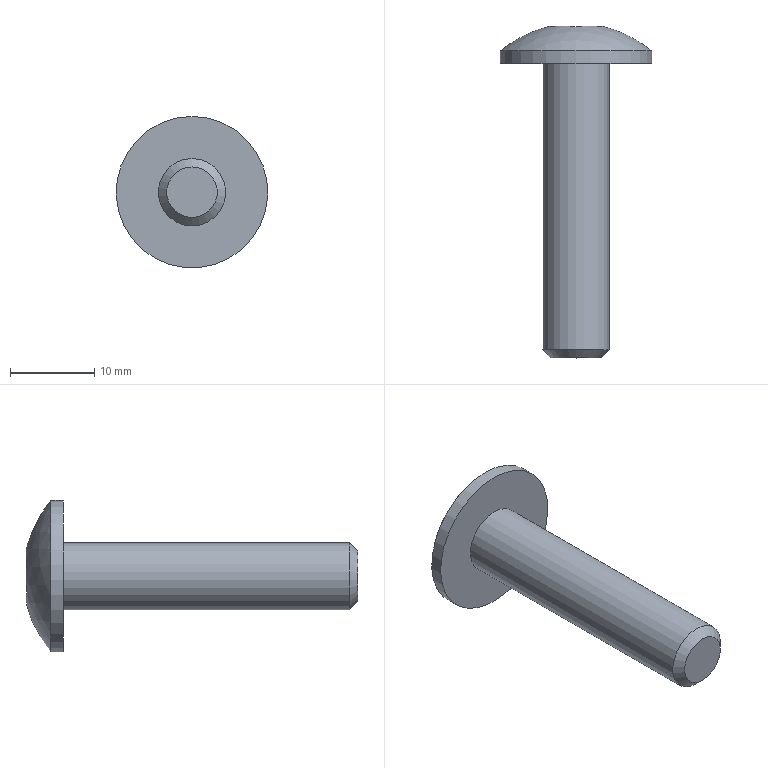Part | STEP file | PN_0012 | 1 solid | 13 faces | box 18 x 39.451 x 18 mm | volume 2453 mm3 | plane 9 | cylinder 2 | sphere 1 | cone 1 | commonest cylinder face diameters 8 x1 18 x1
STEP:
#1=CARTESIAN_POINT('',(0.,0.,0.));
#2=DIRECTION('',(0.,0.,1.));
#3=DIRECTION('',(1.,0.,0.));
#4=AXIS2_PLACEMENT_3D('',#1,#2,#3);
#5=CARTESIAN_POINT('',(0.,0.,9.));
#6=VERTEX_POINT('',#5);
#7=CARTESIAN_POINT('',(0.,0.,0.));
#8=DIRECTION('',(0.,1.,0.));
#9=DIRECTION('',(0.,0.,1.));
#10=AXIS2_PLACEMENT_3D('',#7,#8,#9);
#11=CIRCLE('',#10,9.);
#12=CARTESIAN_POINT('',(0.,0.,0.));
#13=DIRECTION('',(0.,1.,0.));
#14=DIRECTION('',(0.,0.,1.));
#15=AXIS2_PLACEMENT_3D('',#12,#13,#14);
#16=PLANE('',#15);
#17=CARTESIAN_POINT('',(0.,0.));
#18=DIRECTION('',(1.,0.));
#19=AXIS2_PLACEMENT_2D('',#17,#18);
#20=CIRCLE('',#19,9.);
#21=(GEOMETRIC_REPRESENTATION_CONTEXT(2)PARAMETRIC_REPRESENTATION_CONTEXT()REPRESENTATION_CONTEXT('',''));
#22=DEFINITIONAL_REPRESENTATION('',(#20),#21);
#23=PCURVE('',#16,#22);
#24=CARTESIAN_POINT('',(0.,70.,0.));
#25=DIRECTION('',(0.,1.,0.));
#26=DIRECTION('',(0.,0.,1.));
#27=AXIS2_PLACEMENT_3D('',#24,#25,#26);
#28=CYLINDRICAL_SURFACE('',#27,9.);
#29=CARTESIAN_POINT('',(0.,-70.));
#30=DIRECTION('',(1.,0.));
#31=VECTOR('',#30,1.);
#32=LINE('',#29,#31);
#33=(GEOMETRIC_REPRESENTATION_CONTEXT(2)PARAMETRIC_REPRESENTATION_CONTEXT()REPRESENTATION_CONTEXT('',''));
#34=DEFINITIONAL_REPRESENTATION('',(#32),#33);
#35=PCURVE('',#28,#34);
#36=SURFACE_CURVE('',#11,(#23,#35),.PCURVE_S1.);
#37=EDGE_CURVE('',#6,#6,#36,.T.);
#38=ORIENTED_EDGE('',*,*,#37,.F.);
#39=EDGE_LOOP('',(#38));
#40=FACE_BOUND('',#39,.T.);
#41=CARTESIAN_POINT('',(0.,0.,4.));
#42=VERTEX_POINT('',#41);
#43=CARTESIAN_POINT('',(0.,0.,0.));
#44=DIRECTION('',(0.,-1.,0.));
#45=DIRECTION('',(0.,0.,1.));
#46=AXIS2_PLACEMENT_3D('',#43,#44,#45);
#47=CIRCLE('',#46,4.);
#48=CARTESIAN_POINT('',(4.,0.));
#49=CARTESIAN_POINT('',(4.,-6.928));
#50=CARTESIAN_POINT('',(-2.,-3.464));
#51=CARTESIAN_POINT('',(-8.,0.));
#52=CARTESIAN_POINT('',(-2.,3.464));
#53=CARTESIAN_POINT('',(4.,6.928));
#54=CARTESIAN_POINT('',(4.,0.));
#55=(BOUNDED_CURVE()B_SPLINE_CURVE(2,(#48,#49,#50,#51,#52,#53,#54),.UNSPECIFIED.,.T.,.F.)B_SPLINE_CURVE_WITH_KNOTS((1,2,2,2,2,1),(-2.094,0.,2.094,4.189,6.283,8.378),.UNSPECIFIED.)CURVE()GEOMETRIC_REPRESENTATION_ITEM()RATIONAL_B_SPLINE_CURVE((1.,0.5,1.,0.5,1.,0.5,1.))REPRESENTATION_ITEM(''));
#56=(GEOMETRIC_REPRESENTATION_CONTEXT(2)PARAMETRIC_REPRESENTATION_CONTEXT()REPRESENTATION_CONTEXT('',''));
#57=DEFINITIONAL_REPRESENTATION('',(#55),#56);
#58=PCURVE('',#16,#57);
#59=CARTESIAN_POINT('',(0.,-35.,0.));
#60=DIRECTION('',(0.,1.,0.));
#61=DIRECTION('',(0.,0.,1.));
#62=AXIS2_PLACEMENT_3D('',#59,#60,#61);
#63=CYLINDRICAL_SURFACE('',#62,4.);
#64=CARTESIAN_POINT('',(6.283,35.));
#65=DIRECTION('',(-1.,0.));
#66=VECTOR('',#65,1.);
#67=LINE('',#64,#66);
#68=(GEOMETRIC_REPRESENTATION_CONTEXT(2)PARAMETRIC_REPRESENTATION_CONTEXT()REPRESENTATION_CONTEXT('',''));
#69=DEFINITIONAL_REPRESENTATION('',(#67),#68);
#70=PCURVE('',#63,#69);
#71=SURFACE_CURVE('',#47,(#58,#70),.PCURVE_S1.);
#72=EDGE_CURVE('',#42,#42,#71,.T.);
#73=ORIENTED_EDGE('',*,*,#72,.F.);
#74=EDGE_LOOP('',(#73));
#75=FACE_BOUND('',#74,.T.);
#76=ADVANCED_FACE('',(#40,#75),#16,.F.);
#77=CARTESIAN_POINT('',(0.,1.5,9.));
#78=VERTEX_POINT('',#77);
#79=CARTESIAN_POINT('',(0.,1.5,0.));
#80=DIRECTION('',(0.,1.,0.));
#81=DIRECTION('',(0.,0.,1.));
#82=AXIS2_PLACEMENT_3D('',#79,#80,#81);
#83=CIRCLE('',#82,9.);
#84=CARTESIAN_POINT('',(0.,-9.224,0.));
#85=DIRECTION('',(0.,0.,-1.));
#86=DIRECTION('',(1.,0.,0.));
#87=AXIS2_PLACEMENT_3D('',#84,#85,#86);
#88=SPHERICAL_SURFACE('',#87,14.);
#89=CARTESIAN_POINT('',(4.712,-0.6982));
#90=CARTESIAN_POINT('',(4.794,-0.6988));
#91=CARTESIAN_POINT('',(4.951,-0.6746));
#92=CARTESIAN_POINT('',(5.148,-0.5787));
#93=CARTESIAN_POINT('',(5.286,-0.4389));
#94=CARTESIAN_POINT('',(5.372,-0.2727));
#95=CARTESIAN_POINT('',(5.412,-0.09234));
#96=CARTESIAN_POINT('',(5.412,0.09234));
#97=CARTESIAN_POINT('',(5.372,0.2727));
#98=CARTESIAN_POINT('',(5.286,0.439));
#99=CARTESIAN_POINT('',(5.148,0.5786));
#100=CARTESIAN_POINT('',(4.952,0.6749));
#101=CARTESIAN_POINT('',(4.712,0.7099));
#102=CARTESIAN_POINT('',(4.473,0.6749));
#103=CARTESIAN_POINT('',(4.277,0.5786));
#104=CARTESIAN_POINT('',(4.138,0.439));
#105=CARTESIAN_POINT('',(4.053,0.2727));
#106=CARTESIAN_POINT('',(4.012,0.09234));
#107=CARTESIAN_POINT('',(4.012,-0.09234));
#108=CARTESIAN_POINT('',(4.053,-0.2727));
#109=CARTESIAN_POINT('',(4.138,-0.4389));
#110=CARTESIAN_POINT('',(4.277,-0.5787));
#111=CARTESIAN_POINT('',(4.474,-0.6746));
#112=CARTESIAN_POINT('',(4.63,-0.6988));
#113=CARTESIAN_POINT('',(4.712,-0.6982));
#114=B_SPLINE_CURVE_WITH_KNOTS('',3,(#89,#90,#91,#92,#93,#94,#95,#96,#97,#98,#99,#100,#101,#102,#103,#104,#105,#106,#107,#108,#109,#110,#111,#112,#113),.UNSPECIFIED.,.T.,.F.,(4,1,1,1,1,1,1,1,1,1,1,1,1,1,1,1,1,1,1,1,1,1,4),(0.,0.2856,0.5712,0.8568,1.142,1.428,1.714,1.999,2.285,2.57,2.856,3.142,3.427,3.713,3.998,4.284,4.57,4.855,5.141,5.426,5.712,5.998,6.283),.QUASI_UNIFORM_KNOTS.);
#115=(GEOMETRIC_REPRESENTATION_CONTEXT(2)PARAMETRIC_REPRESENTATION_CONTEXT()REPRESENTATION_CONTEXT('',''));
#116=DEFINITIONAL_REPRESENTATION('',(#114),#115);
#117=PCURVE('',#88,#116);
#118=CARTESIAN_POINT('',(0.,-68.5));
#119=DIRECTION('',(1.,0.));
#120=VECTOR('',#119,1.);
#121=LINE('',#118,#120);
#122=(GEOMETRIC_REPRESENTATION_CONTEXT(2)PARAMETRIC_REPRESENTATION_CONTEXT()REPRESENTATION_CONTEXT('',''));
#123=DEFINITIONAL_REPRESENTATION('',(#121),#122);
#124=PCURVE('',#28,#123);
#125=SURFACE_CURVE('',#83,(#117,#124),.PCURVE_S1.);
#126=EDGE_CURVE('',#78,#78,#125,.T.);
#127=ORIENTED_EDGE('',*,*,#126,.T.);
#128=EDGE_LOOP('',(#127));
#129=FACE_BOUND('',#128,.T.);
#130=CARTESIAN_POINT('',(0.,4.341,-3.464));
#131=VERTEX_POINT('',#130);
#132=CARTESIAN_POINT('',(-3.,4.341,-1.732));
#133=VERTEX_POINT('',#132);
#134=CARTESIAN_POINT('',(-1.5,-9.224,-2.598));
#135=DIRECTION('',(0.5,0.,0.866));
#136=DIRECTION('',(0.866,0.,-0.5));
#137=AXIS2_PLACEMENT_3D('',#134,#135,#136);
#138=CIRCLE('',#137,13.675);
#139=CARTESIAN_POINT('',(4.712,0.25));
#140=CARTESIAN_POINT('',(4.709,0.2481));
#141=CARTESIAN_POINT('',(4.702,0.2443));
#142=CARTESIAN_POINT('',(4.692,0.2385));
#143=CARTESIAN_POINT('',(4.682,0.2327));
#144=CARTESIAN_POINT('',(4.673,0.2269));
#145=CARTESIAN_POINT('',(4.663,0.2212));
#146=CARTESIAN_POINT('',(4.653,0.2154));
#147=CARTESIAN_POINT('',(4.643,0.2097));
#148=CARTESIAN_POINT('',(4.633,0.2039));
#149=CARTESIAN_POINT('',(4.623,0.1981));
#150=CARTESIAN_POINT('',(4.613,0.1924));
#151=CARTESIAN_POINT('',(4.603,0.1867));
#152=CARTESIAN_POINT('',(4.593,0.1809));
#153=CARTESIAN_POINT('',(4.583,0.1752));
#154=CARTESIAN_POINT('',(4.574,0.1695));
#155=CARTESIAN_POINT('',(4.564,0.1638));
#156=CARTESIAN_POINT('',(4.554,0.1581));
#157=CARTESIAN_POINT('',(4.544,0.1524));
#158=CARTESIAN_POINT('',(4.534,0.1467));
#159=CARTESIAN_POINT('',(4.524,0.141));
#160=CARTESIAN_POINT('',(4.514,0.1353));
#161=CARTESIAN_POINT('',(4.505,0.1297));
#162=CARTESIAN_POINT('',(4.498,0.1259));
#163=CARTESIAN_POINT('',(4.495,0.124));
#164=B_SPLINE_CURVE_WITH_KNOTS('',3,(#139,#140,#141,#142,#143,#144,#145,#146,#147,#148,#149,#150,#151,#152,#153,#154,#155,#156,#157,#158,#159,#160,#161,#162,#163),.UNSPECIFIED.,.F.,.F.,(4,1,1,1,1,1,1,1,1,1,1,1,1,1,1,1,1,1,1,1,1,1,4),(1.444,1.455,1.467,1.478,1.49,1.502,1.513,1.525,1.536,1.548,1.559,1.571,1.582,1.594,1.605,1.617,1.629,1.64,1.652,1.663,1.675,1.686,1.698),.QUASI_UNIFORM_KNOTS.);
#165=(GEOMETRIC_REPRESENTATION_CONTEXT(2)PARAMETRIC_REPRESENTATION_CONTEXT()REPRESENTATION_CONTEXT('',''));
#166=DEFINITIONAL_REPRESENTATION('',(#164),#165);
#167=PCURVE('',#88,#166);
#168=CARTESIAN_POINT('',(-3.,1.,-1.732));
#169=DIRECTION('',(0.5,0.,0.866));
#170=DIRECTION('',(0.866,0.,-0.5));
#171=AXIS2_PLACEMENT_3D('',#168,#169,#170);
#172=PLANE('',#171);
#173=CARTESIAN_POINT('',(1.732,-10.224));
#174=DIRECTION('',(1.,0.));
#175=AXIS2_PLACEMENT_2D('',#173,#174);
#176=CIRCLE('',#175,13.675);
#177=(GEOMETRIC_REPRESENTATION_CONTEXT(2)PARAMETRIC_REPRESENTATION_CONTEXT()REPRESENTATION_CONTEXT('',''));
#178=DEFINITIONAL_REPRESENTATION('',(#176),#177);
#179=PCURVE('',#172,#178);
#180=SURFACE_CURVE('',#138,(#167,#179),.PCURVE_S1.);
#181=EDGE_CURVE('',#131,#133,#180,.T.);
#182=ORIENTED_EDGE('',*,*,#181,.F.);
#183=CARTESIAN_POINT('',(3.,4.341,-1.732));
#184=VERTEX_POINT('',#183);
#185=CARTESIAN_POINT('',(1.5,-9.224,-2.598));
#186=DIRECTION('',(-0.5,0.,0.866));
#187=DIRECTION('',(0.866,0.,0.5));
#188=AXIS2_PLACEMENT_3D('',#185,#186,#187);
#189=CIRCLE('',#188,13.675);
#190=CARTESIAN_POINT('',(4.93,0.124));
#191=CARTESIAN_POINT('',(4.927,0.1259));
#192=CARTESIAN_POINT('',(4.92,0.1297));
#193=CARTESIAN_POINT('',(4.91,0.1353));
#194=CARTESIAN_POINT('',(4.901,0.141));
#195=CARTESIAN_POINT('',(4.891,0.1467));
#196=CARTESIAN_POINT('',(4.881,0.1524));
#197=CARTESIAN_POINT('',(4.871,0.1581));
#198=CARTESIAN_POINT('',(4.861,0.1638));
#199=CARTESIAN_POINT('',(4.851,0.1695));
#200=CARTESIAN_POINT('',(4.841,0.1752));
#201=CARTESIAN_POINT('',(4.832,0.1809));
#202=CARTESIAN_POINT('',(4.822,0.1867));
#203=CARTESIAN_POINT('',(4.812,0.1924));
#204=CARTESIAN_POINT('',(4.802,0.1981));
#205=CARTESIAN_POINT('',(4.792,0.2039));
#206=CARTESIAN_POINT('',(4.782,0.2097));
#207=CARTESIAN_POINT('',(4.772,0.2154));
#208=CARTESIAN_POINT('',(4.762,0.2212));
#209=CARTESIAN_POINT('',(4.752,0.2269));
#210=CARTESIAN_POINT('',(4.742,0.2327));
#211=CARTESIAN_POINT('',(4.732,0.2385));
#212=CARTESIAN_POINT('',(4.722,0.2443));
#213=CARTESIAN_POINT('',(4.716,0.2481));
#214=CARTESIAN_POINT('',(4.712,0.25));
#215=B_SPLINE_CURVE_WITH_KNOTS('',3,(#190,#191,#192,#193,#194,#195,#196,#197,#198,#199,#200,#201,#202,#203,#204,#205,#206,#207,#208,#209,#210,#211,#212,#213,#214),.UNSPECIFIED.,.F.,.F.,(4,1,1,1,1,1,1,1,1,1,1,1,1,1,1,1,1,1,1,1,1,1,4),(1.444,1.455,1.467,1.478,1.49,1.502,1.513,1.525,1.536,1.548,1.559,1.571,1.582,1.594,1.605,1.617,1.629,1.64,1.652,1.663,1.675,1.686,1.698),.QUASI_UNIFORM_KNOTS.);
#216=(GEOMETRIC_REPRESENTATION_CONTEXT(2)PARAMETRIC_REPRESENTATION_CONTEXT()REPRESENTATION_CONTEXT('',''));
#217=DEFINITIONAL_REPRESENTATION('',(#215),#216);
#218=PCURVE('',#88,#217);
#219=CARTESIAN_POINT('',(0.,1.,-3.464));
#220=DIRECTION('',(-0.5,0.,0.866));
#221=DIRECTION('',(0.866,0.,0.5));
#222=AXIS2_PLACEMENT_3D('',#219,#220,#221);
#223=PLANE('',#222);
#224=CARTESIAN_POINT('',(1.732,-10.224));
#225=DIRECTION('',(1.,0.));
#226=AXIS2_PLACEMENT_2D('',#224,#225);
#227=CIRCLE('',#226,13.675);
#228=(GEOMETRIC_REPRESENTATION_CONTEXT(2)PARAMETRIC_REPRESENTATION_CONTEXT()REPRESENTATION_CONTEXT('',''));
#229=DEFINITIONAL_REPRESENTATION('',(#227),#228);
#230=PCURVE('',#223,#229);
#231=SURFACE_CURVE('',#189,(#218,#230),.PCURVE_S1.);
#232=EDGE_CURVE('',#184,#131,#231,.T.);
#233=ORIENTED_EDGE('',*,*,#232,.F.);
#234=CARTESIAN_POINT('',(3.,4.341,1.732));
#235=VERTEX_POINT('',#234);
#236=CARTESIAN_POINT('',(3.,-9.224,0.));
#237=DIRECTION('',(-1.,0.,0.));
#238=DIRECTION('',(0.,0.,1.));
#239=AXIS2_PLACEMENT_3D('',#236,#237,#238);
#240=CIRCLE('',#239,13.675);
#241=CARTESIAN_POINT('',(4.93,-0.124));
#242=CARTESIAN_POINT('',(4.93,-0.1203));
#243=CARTESIAN_POINT('',(4.93,-0.1128));
#244=CARTESIAN_POINT('',(4.929,-0.1015));
#245=CARTESIAN_POINT('',(4.929,-0.09021));
#246=CARTESIAN_POINT('',(4.929,-0.07894));
#247=CARTESIAN_POINT('',(4.929,-0.06766));
#248=CARTESIAN_POINT('',(4.929,-0.05639));
#249=CARTESIAN_POINT('',(4.929,-0.04511));
#250=CARTESIAN_POINT('',(4.928,-0.03383));
#251=CARTESIAN_POINT('',(4.928,-0.02255));
#252=CARTESIAN_POINT('',(4.928,-0.01128));
#253=CARTESIAN_POINT('',(4.928,0.));
#254=CARTESIAN_POINT('',(4.928,0.01128));
#255=CARTESIAN_POINT('',(4.928,0.02255));
#256=CARTESIAN_POINT('',(4.928,0.03383));
#257=CARTESIAN_POINT('',(4.929,0.04511));
#258=CARTESIAN_POINT('',(4.929,0.05639));
#259=CARTESIAN_POINT('',(4.929,0.06766));
#260=CARTESIAN_POINT('',(4.929,0.07894));
#261=CARTESIAN_POINT('',(4.929,0.09021));
#262=CARTESIAN_POINT('',(4.929,0.1015));
#263=CARTESIAN_POINT('',(4.93,0.1128));
#264=CARTESIAN_POINT('',(4.93,0.1203));
#265=CARTESIAN_POINT('',(4.93,0.124));
#266=B_SPLINE_CURVE_WITH_KNOTS('',3,(#241,#242,#243,#244,#245,#246,#247,#248,#249,#250,#251,#252,#253,#254,#255,#256,#257,#258,#259,#260,#261,#262,#263,#264,#265),.UNSPECIFIED.,.F.,.F.,(4,1,1,1,1,1,1,1,1,1,1,1,1,1,1,1,1,1,1,1,1,1,4),(1.444,1.455,1.467,1.478,1.49,1.502,1.513,1.525,1.536,1.548,1.559,1.571,1.582,1.594,1.605,1.617,1.629,1.64,1.652,1.663,1.675,1.686,1.698),.QUASI_UNIFORM_KNOTS.);
#267=(GEOMETRIC_REPRESENTATION_CONTEXT(2)PARAMETRIC_REPRESENTATION_CONTEXT()REPRESENTATION_CONTEXT('',''));
#268=DEFINITIONAL_REPRESENTATION('',(#266),#267);
#269=PCURVE('',#88,#268);
#270=CARTESIAN_POINT('',(3.,1.,-1.732));
#271=DIRECTION('',(-1.,0.,0.));
#272=DIRECTION('',(0.,0.,1.));
#273=AXIS2_PLACEMENT_3D('',#270,#271,#272);
#274=PLANE('',#273);
#275=CARTESIAN_POINT('',(1.732,-10.224));
#276=DIRECTION('',(1.,0.));
#277=AXIS2_PLACEMENT_2D('',#275,#276);
#278=CIRCLE('',#277,13.675);
#279=(GEOMETRIC_REPRESENTATION_CONTEXT(2)PARAMETRIC_REPRESENTATION_CONTEXT()REPRESENTATION_CONTEXT('',''));
#280=DEFINITIONAL_REPRESENTATION('',(#278),#279);
#281=PCURVE('',#274,#280);
#282=SURFACE_CURVE('',#240,(#269,#281),.PCURVE_S1.);
#283=EDGE_CURVE('',#235,#184,#282,.T.);
#284=ORIENTED_EDGE('',*,*,#283,.F.);
#285=CARTESIAN_POINT('',(0.,4.341,3.464));
#286=VERTEX_POINT('',#285);
#287=CARTESIAN_POINT('',(1.5,-9.224,2.598));
#288=DIRECTION('',(-0.5,0.,-0.866));
#289=DIRECTION('',(-0.866,0.,0.5));
#290=AXIS2_PLACEMENT_3D('',#287,#288,#289);
#291=CIRCLE('',#290,13.675);
#292=CARTESIAN_POINT('',(4.712,-0.25));
#293=CARTESIAN_POINT('',(4.716,-0.2481));
#294=CARTESIAN_POINT('',(4.722,-0.2443));
#295=CARTESIAN_POINT('',(4.732,-0.2385));
#296=CARTESIAN_POINT('',(4.742,-0.2327));
#297=CARTESIAN_POINT('',(4.752,-0.2269));
#298=CARTESIAN_POINT('',(4.762,-0.2212));
#299=CARTESIAN_POINT('',(4.772,-0.2154));
#300=CARTESIAN_POINT('',(4.782,-0.2097));
#301=CARTESIAN_POINT('',(4.792,-0.2039));
#302=CARTESIAN_POINT('',(4.802,-0.1981));
#303=CARTESIAN_POINT('',(4.812,-0.1924));
#304=CARTESIAN_POINT('',(4.822,-0.1867));
#305=CARTESIAN_POINT('',(4.832,-0.1809));
#306=CARTESIAN_POINT('',(4.841,-0.1752));
#307=CARTESIAN_POINT('',(4.851,-0.1695));
#308=CARTESIAN_POINT('',(4.861,-0.1638));
#309=CARTESIAN_POINT('',(4.871,-0.1581));
#310=CARTESIAN_POINT('',(4.881,-0.1524));
#311=CARTESIAN_POINT('',(4.891,-0.1467));
#312=CARTESIAN_POINT('',(4.901,-0.141));
#313=CARTESIAN_POINT('',(4.91,-0.1353));
#314=CARTESIAN_POINT('',(4.92,-0.1297));
#315=CARTESIAN_POINT('',(4.927,-0.1259));
#316=CARTESIAN_POINT('',(4.93,-0.124));
#317=B_SPLINE_CURVE_WITH_KNOTS('',3,(#292,#293,#294,#295,#296,#297,#298,#299,#300,#301,#302,#303,#304,#305,#306,#307,#308,#309,#310,#311,#312,#313,#314,#315,#316),.UNSPECIFIED.,.F.,.F.,(4,1,1,1,1,1,1,1,1,1,1,1,1,1,1,1,1,1,1,1,1,1,4),(1.444,1.455,1.467,1.478,1.49,1.502,1.513,1.525,1.536,1.548,1.559,1.571,1.582,1.594,1.605,1.617,1.629,1.64,1.652,1.663,1.675,1.686,1.698),.QUASI_UNIFORM_KNOTS.);
#318=(GEOMETRIC_REPRESENTATION_CONTEXT(2)PARAMETRIC_REPRESENTATION_CONTEXT()REPRESENTATION_CONTEXT('',''));
#319=DEFINITIONAL_REPRESENTATION('',(#317),#318);
#320=PCURVE('',#88,#319);
#321=CARTESIAN_POINT('',(3.,1.,1.732));
#322=DIRECTION('',(-0.5,0.,-0.866));
#323=DIRECTION('',(-0.866,0.,0.5));
#324=AXIS2_PLACEMENT_3D('',#321,#322,#323);
#325=PLANE('',#324);
#326=CARTESIAN_POINT('',(1.732,-10.224));
#327=DIRECTION('',(1.,0.));
#328=AXIS2_PLACEMENT_2D('',#326,#327);
#329=CIRCLE('',#328,13.675);
#330=(GEOMETRIC_REPRESENTATION_CONTEXT(2)PARAMETRIC_REPRESENTATION_CONTEXT()REPRESENTATION_CONTEXT('',''));
#331=DEFINITIONAL_REPRESENTATION('',(#329),#330);
#332=PCURVE('',#325,#331);
#333=SURFACE_CURVE('',#291,(#320,#332),.PCURVE_S1.);
#334=EDGE_CURVE('',#286,#235,#333,.T.);
#335=ORIENTED_EDGE('',*,*,#334,.F.);
#336=CARTESIAN_POINT('',(-3.,4.341,1.732));
#337=VERTEX_POINT('',#336);
#338=CARTESIAN_POINT('',(-1.5,-9.224,2.598));
#339=DIRECTION('',(0.5,0.,-0.866));
#340=DIRECTION('',(-0.866,0.,-0.5));
#341=AXIS2_PLACEMENT_3D('',#338,#339,#340);
#342=CIRCLE('',#341,13.675);
#343=CARTESIAN_POINT('',(4.495,-0.124));
#344=CARTESIAN_POINT('',(4.498,-0.1259));
#345=CARTESIAN_POINT('',(4.505,-0.1297));
#346=CARTESIAN_POINT('',(4.514,-0.1353));
#347=CARTESIAN_POINT('',(4.524,-0.141));
#348=CARTESIAN_POINT('',(4.534,-0.1467));
#349=CARTESIAN_POINT('',(4.544,-0.1524));
#350=CARTESIAN_POINT('',(4.554,-0.1581));
#351=CARTESIAN_POINT('',(4.564,-0.1638));
#352=CARTESIAN_POINT('',(4.574,-0.1695));
#353=CARTESIAN_POINT('',(4.583,-0.1752));
#354=CARTESIAN_POINT('',(4.593,-0.1809));
#355=CARTESIAN_POINT('',(4.603,-0.1867));
#356=CARTESIAN_POINT('',(4.613,-0.1924));
#357=CARTESIAN_POINT('',(4.623,-0.1981));
#358=CARTESIAN_POINT('',(4.633,-0.2039));
#359=CARTESIAN_POINT('',(4.643,-0.2097));
#360=CARTESIAN_POINT('',(4.653,-0.2154));
#361=CARTESIAN_POINT('',(4.663,-0.2212));
#362=CARTESIAN_POINT('',(4.673,-0.2269));
#363=CARTESIAN_POINT('',(4.682,-0.2327));
#364=CARTESIAN_POINT('',(4.692,-0.2385));
#365=CARTESIAN_POINT('',(4.702,-0.2443));
#366=CARTESIAN_POINT('',(4.709,-0.2481));
#367=CARTESIAN_POINT('',(4.712,-0.25));
#368=B_SPLINE_CURVE_WITH_KNOTS('',3,(#343,#344,#345,#346,#347,#348,#349,#350,#351,#352,#353,#354,#355,#356,#357,#358,#359,#360,#361,#362,#363,#364,#365,#366,#367),.UNSPECIFIED.,.F.,.F.,(4,1,1,1,1,1,1,1,1,1,1,1,1,1,1,1,1,1,1,1,1,1,4),(1.444,1.455,1.467,1.478,1.49,1.502,1.513,1.525,1.536,1.548,1.559,1.571,1.582,1.594,1.605,1.617,1.629,1.64,1.652,1.663,1.675,1.686,1.698),.QUASI_UNIFORM_KNOTS.);
#369=(GEOMETRIC_REPRESENTATION_CONTEXT(2)PARAMETRIC_REPRESENTATION_CONTEXT()REPRESENTATION_CONTEXT('',''));
#370=DEFINITIONAL_REPRESENTATION('',(#368),#369);
#371=PCURVE('',#88,#370);
#372=CARTESIAN_POINT('',(0.,1.,3.464));
#373=DIRECTION('',(0.5,0.,-0.866));
#374=DIRECTION('',(-0.866,0.,-0.5));
#375=AXIS2_PLACEMENT_3D('',#372,#373,#374);
#376=PLANE('',#375);
#377=CARTESIAN_POINT('',(1.732,-10.224));
#378=DIRECTION('',(1.,0.));
#379=AXIS2_PLACEMENT_2D('',#377,#378);
#380=CIRCLE('',#379,13.675);
#381=(GEOMETRIC_REPRESENTATION_CONTEXT(2)PARAMETRIC_REPRESENTATION_CONTEXT()REPRESENTATION_CONTEXT('',''));
#382=DEFINITIONAL_REPRESENTATION('',(#380),#381);
#383=PCURVE('',#376,#382);
#384=SURFACE_CURVE('',#342,(#371,#383),.PCURVE_S1.);
#385=EDGE_CURVE('',#337,#286,#384,.T.);
#386=ORIENTED_EDGE('',*,*,#385,.F.);
#387=CARTESIAN_POINT('',(-3.,-9.224,0.));
#388=DIRECTION('',(1.,0.,0.));
#389=DIRECTION('',(0.,0.,-1.));
#390=AXIS2_PLACEMENT_3D('',#387,#388,#389);
#391=CIRCLE('',#390,13.675);
#392=CARTESIAN_POINT('',(4.495,0.124));
#393=CARTESIAN_POINT('',(4.495,0.1203));
#394=CARTESIAN_POINT('',(4.495,0.1128));
#395=CARTESIAN_POINT('',(4.495,0.1015));
#396=CARTESIAN_POINT('',(4.496,0.09021));
#397=CARTESIAN_POINT('',(4.496,0.07894));
#398=CARTESIAN_POINT('',(4.496,0.06766));
#399=CARTESIAN_POINT('',(4.496,0.05639));
#400=CARTESIAN_POINT('',(4.496,0.04511));
#401=CARTESIAN_POINT('',(4.496,0.03383));
#402=CARTESIAN_POINT('',(4.496,0.02255));
#403=CARTESIAN_POINT('',(4.496,0.01128));
#404=CARTESIAN_POINT('',(4.496,0.));
#405=CARTESIAN_POINT('',(4.496,-0.01128));
#406=CARTESIAN_POINT('',(4.496,-0.02255));
#407=CARTESIAN_POINT('',(4.496,-0.03383));
#408=CARTESIAN_POINT('',(4.496,-0.04511));
#409=CARTESIAN_POINT('',(4.496,-0.05639));
#410=CARTESIAN_POINT('',(4.496,-0.06766));
#411=CARTESIAN_POINT('',(4.496,-0.07894));
#412=CARTESIAN_POINT('',(4.496,-0.09021));
#413=CARTESIAN_POINT('',(4.495,-0.1015));
#414=CARTESIAN_POINT('',(4.495,-0.1128));
#415=CARTESIAN_POINT('',(4.495,-0.1203));
#416=CARTESIAN_POINT('',(4.495,-0.124));
#417=B_SPLINE_CURVE_WITH_KNOTS('',3,(#392,#393,#394,#395,#396,#397,#398,#399,#400,#401,#402,#403,#404,#405,#406,#407,#408,#409,#410,#411,#412,#413,#414,#415,#416),.UNSPECIFIED.,.F.,.F.,(4,1,1,1,1,1,1,1,1,1,1,1,1,1,1,1,1,1,1,1,1,1,4),(1.444,1.455,1.467,1.478,1.49,1.502,1.513,1.525,1.536,1.548,1.559,1.571,1.582,1.594,1.605,1.617,1.629,1.64,1.652,1.663,1.675,1.686,1.698),.QUASI_UNIFORM_KNOTS.);
#418=(GEOMETRIC_REPRESENTATION_CONTEXT(2)PARAMETRIC_REPRESENTATION_CONTEXT()REPRESENTATION_CONTEXT('',''));
#419=DEFINITIONAL_REPRESENTATION('',(#417),#418);
#420=PCURVE('',#88,#419);
#421=CARTESIAN_POINT('',(-3.,1.,1.732));
#422=DIRECTION('',(1.,0.,0.));
#423=DIRECTION('',(0.,0.,-1.));
#424=AXIS2_PLACEMENT_3D('',#421,#422,#423);
#425=PLANE('',#424);
#426=CARTESIAN_POINT('',(1.732,-10.224));
#427=DIRECTION('',(1.,0.));
#428=AXIS2_PLACEMENT_2D('',#426,#427);
#429=CIRCLE('',#428,13.675);
#430=(GEOMETRIC_REPRESENTATION_CONTEXT(2)PARAMETRIC_REPRESENTATION_CONTEXT()REPRESENTATION_CONTEXT('',''));
#431=DEFINITIONAL_REPRESENTATION('',(#429),#430);
#432=PCURVE('',#425,#431);
#433=SURFACE_CURVE('',#391,(#420,#432),.PCURVE_S1.);
#434=EDGE_CURVE('',#133,#337,#433,.T.);
#435=ORIENTED_EDGE('',*,*,#434,.F.);
#436=EDGE_LOOP('',(#182,#233,#284,#335,#386,#435));
#437=FACE_BOUND('',#436,.T.);
#438=ADVANCED_FACE('',(#129,#437),#88,.T.);
#439=ORIENTED_EDGE('',*,*,#126,.F.);
#440=CARTESIAN_POINT('',(0.,0.,9.));
#441=CARTESIAN_POINT('',(0.,1.5,9.));
#442=B_SPLINE_CURVE_WITH_KNOTS('',1,(#440,#441),.UNSPECIFIED.,.F.,.F.,(2,2),(-70.,-68.5),.PIECEWISE_BEZIER_KNOTS.);
#443=CARTESIAN_POINT('',(0.,0.));
#444=DIRECTION('',(0.,1.));
#445=VECTOR('',#444,1.);
#446=LINE('',#443,#445);
#447=(GEOMETRIC_REPRESENTATION_CONTEXT(2)PARAMETRIC_REPRESENTATION_CONTEXT()REPRESENTATION_CONTEXT('',''));
#448=DEFINITIONAL_REPRESENTATION('',(#446),#447);
#449=PCURVE('',#28,#448);
#450=CARTESIAN_POINT('',(6.283,0.));
#451=DIRECTION('',(0.,1.));
#452=VECTOR('',#451,1.);
#453=LINE('',#450,#452);
#454=(GEOMETRIC_REPRESENTATION_CONTEXT(2)PARAMETRIC_REPRESENTATION_CONTEXT()REPRESENTATION_CONTEXT('',''));
#455=DEFINITIONAL_REPRESENTATION('',(#453),#454);
#456=PCURVE('',#28,#455);
#457=SEAM_CURVE('',#442,(#449,#456),.PCURVE_S1.);
#458=EDGE_CURVE('',#6,#78,#457,.T.);
#459=ORIENTED_EDGE('',*,*,#458,.F.);
#460=ORIENTED_EDGE('',*,*,#37,.T.);
#461=ORIENTED_EDGE('',*,*,#458,.T.);
#462=EDGE_LOOP('',(#439,#459,#460,#461));
#463=FACE_BOUND('',#462,.T.);
#464=ADVANCED_FACE('',(#463),#28,.T.);
#465=ORIENTED_EDGE('',*,*,#181,.T.);
#466=CARTESIAN_POINT('',(-3.,1.,-1.732));
#467=VERTEX_POINT('',#466);
#468=CARTESIAN_POINT('',(-3.,1.,-1.732));
#469=DIRECTION('',(0.,1.,0.));
#470=VECTOR('',#469,1.);
#471=LINE('',#468,#470);
#472=CARTESIAN_POINT('',(0.,0.));
#473=DIRECTION('',(0.,1.));
#474=VECTOR('',#473,1.);
#475=LINE('',#472,#474);
#476=(GEOMETRIC_REPRESENTATION_CONTEXT(2)PARAMETRIC_REPRESENTATION_CONTEXT()REPRESENTATION_CONTEXT('',''));
#477=DEFINITIONAL_REPRESENTATION('',(#475),#476);
#478=PCURVE('',#172,#477);
#479=CARTESIAN_POINT('',(3.464,0.));
#480=DIRECTION('',(0.,1.));
#481=VECTOR('',#480,1.);
#482=LINE('',#479,#481);
#483=(GEOMETRIC_REPRESENTATION_CONTEXT(2)PARAMETRIC_REPRESENTATION_CONTEXT()REPRESENTATION_CONTEXT('',''));
#484=DEFINITIONAL_REPRESENTATION('',(#482),#483);
#485=PCURVE('',#425,#484);
#486=SURFACE_CURVE('',#471,(#478,#485),.PCURVE_S1.);
#487=EDGE_CURVE('',#467,#133,#486,.T.);
#488=ORIENTED_EDGE('',*,*,#487,.F.);
#489=CARTESIAN_POINT('',(0.,1.,-3.464));
#490=VERTEX_POINT('',#489);
#491=CARTESIAN_POINT('',(-3.,1.,-1.732));
#492=DIRECTION('',(0.866,0.,-0.5));
#493=VECTOR('',#492,1.);
#494=LINE('',#491,#493);
#495=CARTESIAN_POINT('',(0.,0.));
#496=DIRECTION('',(1.,0.));
#497=VECTOR('',#496,1.);
#498=LINE('',#495,#497);
#499=(GEOMETRIC_REPRESENTATION_CONTEXT(2)PARAMETRIC_REPRESENTATION_CONTEXT()REPRESENTATION_CONTEXT('',''));
#500=DEFINITIONAL_REPRESENTATION('',(#498),#499);
#501=PCURVE('',#172,#500);
#502=CARTESIAN_POINT('',(-3.,1.,-1.732));
#503=DIRECTION('',(0.,1.,0.));
#504=DIRECTION('',(0.,0.,1.));
#505=AXIS2_PLACEMENT_3D('',#502,#503,#504);
#506=PLANE('',#505);
#507=CARTESIAN_POINT('',(0.,0.));
#508=DIRECTION('',(-0.5,0.866));
#509=VECTOR('',#508,1.);
#510=LINE('',#507,#509);
#511=(GEOMETRIC_REPRESENTATION_CONTEXT(2)PARAMETRIC_REPRESENTATION_CONTEXT()REPRESENTATION_CONTEXT('',''));
#512=DEFINITIONAL_REPRESENTATION('',(#510),#511);
#513=PCURVE('',#506,#512);
#514=SURFACE_CURVE('',#494,(#501,#513),.PCURVE_S1.);
#515=EDGE_CURVE('',#467,#490,#514,.T.);
#516=ORIENTED_EDGE('',*,*,#515,.T.);
#517=CARTESIAN_POINT('',(0.,1.,-3.464));
#518=DIRECTION('',(0.,1.,0.));
#519=VECTOR('',#518,1.);
#520=LINE('',#517,#519);
#521=CARTESIAN_POINT('',(3.464,0.));
#522=DIRECTION('',(0.,1.));
#523=VECTOR('',#522,1.);
#524=LINE('',#521,#523);
#525=(GEOMETRIC_REPRESENTATION_CONTEXT(2)PARAMETRIC_REPRESENTATION_CONTEXT()REPRESENTATION_CONTEXT('',''));
#526=DEFINITIONAL_REPRESENTATION('',(#524),#525);
#527=PCURVE('',#172,#526);
#528=CARTESIAN_POINT('',(0.,0.));
#529=DIRECTION('',(0.,1.));
#530=VECTOR('',#529,1.);
#531=LINE('',#528,#530);
#532=(GEOMETRIC_REPRESENTATION_CONTEXT(2)PARAMETRIC_REPRESENTATION_CONTEXT()REPRESENTATION_CONTEXT('',''));
#533=DEFINITIONAL_REPRESENTATION('',(#531),#532);
#534=PCURVE('',#223,#533);
#535=SURFACE_CURVE('',#520,(#527,#534),.PCURVE_S1.);
#536=EDGE_CURVE('',#490,#131,#535,.T.);
#537=ORIENTED_EDGE('',*,*,#536,.T.);
#538=EDGE_LOOP('',(#465,#488,#516,#537));
#539=FACE_BOUND('',#538,.T.);
#540=ADVANCED_FACE('',(#539),#172,.T.);
#541=ORIENTED_EDGE('',*,*,#232,.T.);
#542=ORIENTED_EDGE('',*,*,#536,.F.);
#543=CARTESIAN_POINT('',(3.,1.,-1.732));
#544=VERTEX_POINT('',#543);
#545=CARTESIAN_POINT('',(0.,1.,-3.464));
#546=DIRECTION('',(0.866,0.,0.5));
#547=VECTOR('',#546,1.);
#548=LINE('',#545,#547);
#549=CARTESIAN_POINT('',(0.,0.));
#550=DIRECTION('',(1.,0.));
#551=VECTOR('',#550,1.);
#552=LINE('',#549,#551);
#553=(GEOMETRIC_REPRESENTATION_CONTEXT(2)PARAMETRIC_REPRESENTATION_CONTEXT()REPRESENTATION_CONTEXT('',''));
#554=DEFINITIONAL_REPRESENTATION('',(#552),#553);
#555=PCURVE('',#223,#554);
#556=CARTESIAN_POINT('',(-1.732,3.));
#557=DIRECTION('',(0.5,0.866));
#558=VECTOR('',#557,1.);
#559=LINE('',#556,#558);
#560=(GEOMETRIC_REPRESENTATION_CONTEXT(2)PARAMETRIC_REPRESENTATION_CONTEXT()REPRESENTATION_CONTEXT('',''));
#561=DEFINITIONAL_REPRESENTATION('',(#559),#560);
#562=PCURVE('',#506,#561);
#563=SURFACE_CURVE('',#548,(#555,#562),.PCURVE_S1.);
#564=EDGE_CURVE('',#490,#544,#563,.T.);
#565=ORIENTED_EDGE('',*,*,#564,.T.);
#566=CARTESIAN_POINT('',(3.,1.,-1.732));
#567=DIRECTION('',(0.,1.,0.));
#568=VECTOR('',#567,1.);
#569=LINE('',#566,#568);
#570=CARTESIAN_POINT('',(3.464,0.));
#571=DIRECTION('',(0.,1.));
#572=VECTOR('',#571,1.);
#573=LINE('',#570,#572);
#574=(GEOMETRIC_REPRESENTATION_CONTEXT(2)PARAMETRIC_REPRESENTATION_CONTEXT()REPRESENTATION_CONTEXT('',''));
#575=DEFINITIONAL_REPRESENTATION('',(#573),#574);
#576=PCURVE('',#223,#575);
#577=CARTESIAN_POINT('',(0.,0.));
#578=DIRECTION('',(0.,1.));
#579=VECTOR('',#578,1.);
#580=LINE('',#577,#579);
#581=(GEOMETRIC_REPRESENTATION_CONTEXT(2)PARAMETRIC_REPRESENTATION_CONTEXT()REPRESENTATION_CONTEXT('',''));
#582=DEFINITIONAL_REPRESENTATION('',(#580),#581);
#583=PCURVE('',#274,#582);
#584=SURFACE_CURVE('',#569,(#576,#583),.PCURVE_S1.);
#585=EDGE_CURVE('',#544,#184,#584,.T.);
#586=ORIENTED_EDGE('',*,*,#585,.T.);
#587=EDGE_LOOP('',(#541,#542,#565,#586));
#588=FACE_BOUND('',#587,.T.);
#589=ADVANCED_FACE('',(#588),#223,.T.);
#590=ORIENTED_EDGE('',*,*,#283,.T.);
#591=ORIENTED_EDGE('',*,*,#585,.F.);
#592=CARTESIAN_POINT('',(3.,1.,1.732));
#593=VERTEX_POINT('',#592);
#594=CARTESIAN_POINT('',(3.,1.,-1.732));
#595=DIRECTION('',(0.,0.,1.));
#596=VECTOR('',#595,1.);
#597=LINE('',#594,#596);
#598=CARTESIAN_POINT('',(0.,0.));
#599=DIRECTION('',(1.,0.));
#600=VECTOR('',#599,1.);
#601=LINE('',#598,#600);
#602=(GEOMETRIC_REPRESENTATION_CONTEXT(2)PARAMETRIC_REPRESENTATION_CONTEXT()REPRESENTATION_CONTEXT('',''));
#603=DEFINITIONAL_REPRESENTATION('',(#601),#602);
#604=PCURVE('',#274,#603);
#605=CARTESIAN_POINT('',(0.,6.));
#606=DIRECTION('',(1.,0.));
#607=VECTOR('',#606,1.);
#608=LINE('',#605,#607);
#609=(GEOMETRIC_REPRESENTATION_CONTEXT(2)PARAMETRIC_REPRESENTATION_CONTEXT()REPRESENTATION_CONTEXT('',''));
#610=DEFINITIONAL_REPRESENTATION('',(#608),#609);
#611=PCURVE('',#506,#610);
#612=SURFACE_CURVE('',#597,(#604,#611),.PCURVE_S1.);
#613=EDGE_CURVE('',#544,#593,#612,.T.);
#614=ORIENTED_EDGE('',*,*,#613,.T.);
#615=CARTESIAN_POINT('',(3.,1.,1.732));
#616=DIRECTION('',(0.,1.,0.));
#617=VECTOR('',#616,1.);
#618=LINE('',#615,#617);
#619=CARTESIAN_POINT('',(3.464,0.));
#620=DIRECTION('',(0.,1.));
#621=VECTOR('',#620,1.);
#622=LINE('',#619,#621);
#623=(GEOMETRIC_REPRESENTATION_CONTEXT(2)PARAMETRIC_REPRESENTATION_CONTEXT()REPRESENTATION_CONTEXT('',''));
#624=DEFINITIONAL_REPRESENTATION('',(#622),#623);
#625=PCURVE('',#274,#624);
#626=CARTESIAN_POINT('',(0.,0.));
#627=DIRECTION('',(0.,1.));
#628=VECTOR('',#627,1.);
#629=LINE('',#626,#628);
#630=(GEOMETRIC_REPRESENTATION_CONTEXT(2)PARAMETRIC_REPRESENTATION_CONTEXT()REPRESENTATION_CONTEXT('',''));
#631=DEFINITIONAL_REPRESENTATION('',(#629),#630);
#632=PCURVE('',#325,#631);
#633=SURFACE_CURVE('',#618,(#625,#632),.PCURVE_S1.);
#634=EDGE_CURVE('',#593,#235,#633,.T.);
#635=ORIENTED_EDGE('',*,*,#634,.T.);
#636=EDGE_LOOP('',(#590,#591,#614,#635));
#637=FACE_BOUND('',#636,.T.);
#638=ADVANCED_FACE('',(#637),#274,.T.);
#639=ORIENTED_EDGE('',*,*,#334,.T.);
#640=ORIENTED_EDGE('',*,*,#634,.F.);
#641=CARTESIAN_POINT('',(0.,1.,3.464));
#642=VERTEX_POINT('',#641);
#643=CARTESIAN_POINT('',(3.,1.,1.732));
#644=DIRECTION('',(-0.866,0.,0.5));
#645=VECTOR('',#644,1.);
#646=LINE('',#643,#645);
#647=CARTESIAN_POINT('',(0.,0.));
#648=DIRECTION('',(1.,0.));
#649=VECTOR('',#648,1.);
#650=LINE('',#647,#649);
#651=(GEOMETRIC_REPRESENTATION_CONTEXT(2)PARAMETRIC_REPRESENTATION_CONTEXT()REPRESENTATION_CONTEXT('',''));
#652=DEFINITIONAL_REPRESENTATION('',(#650),#651);
#653=PCURVE('',#325,#652);
#654=CARTESIAN_POINT('',(3.464,6.));
#655=DIRECTION('',(0.5,-0.866));
#656=VECTOR('',#655,1.);
#657=LINE('',#654,#656);
#658=(GEOMETRIC_REPRESENTATION_CONTEXT(2)PARAMETRIC_REPRESENTATION_CONTEXT()REPRESENTATION_CONTEXT('',''));
#659=DEFINITIONAL_REPRESENTATION('',(#657),#658);
#660=PCURVE('',#506,#659);
#661=SURFACE_CURVE('',#646,(#653,#660),.PCURVE_S1.);
#662=EDGE_CURVE('',#593,#642,#661,.T.);
#663=ORIENTED_EDGE('',*,*,#662,.T.);
#664=CARTESIAN_POINT('',(0.,1.,3.464));
#665=DIRECTION('',(0.,1.,0.));
#666=VECTOR('',#665,1.);
#667=LINE('',#664,#666);
#668=CARTESIAN_POINT('',(3.464,0.));
#669=DIRECTION('',(0.,1.));
#670=VECTOR('',#669,1.);
#671=LINE('',#668,#670);
#672=(GEOMETRIC_REPRESENTATION_CONTEXT(2)PARAMETRIC_REPRESENTATION_CONTEXT()REPRESENTATION_CONTEXT('',''));
#673=DEFINITIONAL_REPRESENTATION('',(#671),#672);
#674=PCURVE('',#325,#673);
#675=CARTESIAN_POINT('',(0.,0.));
#676=DIRECTION('',(0.,1.));
#677=VECTOR('',#676,1.);
#678=LINE('',#675,#677);
#679=(GEOMETRIC_REPRESENTATION_CONTEXT(2)PARAMETRIC_REPRESENTATION_CONTEXT()REPRESENTATION_CONTEXT('',''));
#680=DEFINITIONAL_REPRESENTATION('',(#678),#679);
#681=PCURVE('',#376,#680);
#682=SURFACE_CURVE('',#667,(#674,#681),.PCURVE_S1.);
#683=EDGE_CURVE('',#642,#286,#682,.T.);
#684=ORIENTED_EDGE('',*,*,#683,.T.);
#685=EDGE_LOOP('',(#639,#640,#663,#684));
#686=FACE_BOUND('',#685,.T.);
#687=ADVANCED_FACE('',(#686),#325,.T.);
#688=ORIENTED_EDGE('',*,*,#385,.T.);
#689=ORIENTED_EDGE('',*,*,#683,.F.);
#690=CARTESIAN_POINT('',(-3.,1.,1.732));
#691=VERTEX_POINT('',#690);
#692=CARTESIAN_POINT('',(0.,1.,3.464));
#693=DIRECTION('',(-0.866,0.,-0.5));
#694=VECTOR('',#693,1.);
#695=LINE('',#692,#694);
#696=CARTESIAN_POINT('',(0.,0.));
#697=DIRECTION('',(1.,0.));
#698=VECTOR('',#697,1.);
#699=LINE('',#696,#698);
#700=(GEOMETRIC_REPRESENTATION_CONTEXT(2)PARAMETRIC_REPRESENTATION_CONTEXT()REPRESENTATION_CONTEXT('',''));
#701=DEFINITIONAL_REPRESENTATION('',(#699),#700);
#702=PCURVE('',#376,#701);
#703=CARTESIAN_POINT('',(5.196,3.));
#704=DIRECTION('',(-0.5,-0.866));
#705=VECTOR('',#704,1.);
#706=LINE('',#703,#705);
#707=(GEOMETRIC_REPRESENTATION_CONTEXT(2)PARAMETRIC_REPRESENTATION_CONTEXT()REPRESENTATION_CONTEXT('',''));
#708=DEFINITIONAL_REPRESENTATION('',(#706),#707);
#709=PCURVE('',#506,#708);
#710=SURFACE_CURVE('',#695,(#702,#709),.PCURVE_S1.);
#711=EDGE_CURVE('',#642,#691,#710,.T.);
#712=ORIENTED_EDGE('',*,*,#711,.T.);
#713=CARTESIAN_POINT('',(-3.,1.,1.732));
#714=DIRECTION('',(0.,1.,0.));
#715=VECTOR('',#714,1.);
#716=LINE('',#713,#715);
#717=CARTESIAN_POINT('',(3.464,0.));
#718=DIRECTION('',(0.,1.));
#719=VECTOR('',#718,1.);
#720=LINE('',#717,#719);
#721=(GEOMETRIC_REPRESENTATION_CONTEXT(2)PARAMETRIC_REPRESENTATION_CONTEXT()REPRESENTATION_CONTEXT('',''));
#722=DEFINITIONAL_REPRESENTATION('',(#720),#721);
#723=PCURVE('',#376,#722);
#724=CARTESIAN_POINT('',(0.,0.));
#725=DIRECTION('',(0.,1.));
#726=VECTOR('',#725,1.);
#727=LINE('',#724,#726);
#728=(GEOMETRIC_REPRESENTATION_CONTEXT(2)PARAMETRIC_REPRESENTATION_CONTEXT()REPRESENTATION_CONTEXT('',''));
#729=DEFINITIONAL_REPRESENTATION('',(#727),#728);
#730=PCURVE('',#425,#729);
#731=SURFACE_CURVE('',#716,(#723,#730),.PCURVE_S1.);
#732=EDGE_CURVE('',#691,#337,#731,.T.);
#733=ORIENTED_EDGE('',*,*,#732,.T.);
#734=EDGE_LOOP('',(#688,#689,#712,#733));
#735=FACE_BOUND('',#734,.T.);
#736=ADVANCED_FACE('',(#735),#376,.T.);
#737=ORIENTED_EDGE('',*,*,#434,.T.);
#738=ORIENTED_EDGE('',*,*,#732,.F.);
#739=CARTESIAN_POINT('',(-3.,1.,1.732));
#740=DIRECTION('',(0.,0.,-1.));
#741=VECTOR('',#740,1.);
#742=LINE('',#739,#741);
#743=CARTESIAN_POINT('',(0.,0.));
#744=DIRECTION('',(1.,0.));
#745=VECTOR('',#744,1.);
#746=LINE('',#743,#745);
#747=(GEOMETRIC_REPRESENTATION_CONTEXT(2)PARAMETRIC_REPRESENTATION_CONTEXT()REPRESENTATION_CONTEXT('',''));
#748=DEFINITIONAL_REPRESENTATION('',(#746),#747);
#749=PCURVE('',#425,#748);
#750=CARTESIAN_POINT('',(3.464,0.));
#751=DIRECTION('',(-1.,0.));
#752=VECTOR('',#751,1.);
#753=LINE('',#750,#752);
#754=(GEOMETRIC_REPRESENTATION_CONTEXT(2)PARAMETRIC_REPRESENTATION_CONTEXT()REPRESENTATION_CONTEXT('',''));
#755=DEFINITIONAL_REPRESENTATION('',(#753),#754);
#756=PCURVE('',#506,#755);
#757=SURFACE_CURVE('',#742,(#749,#756),.PCURVE_S1.);
#758=EDGE_CURVE('',#691,#467,#757,.T.);
#759=ORIENTED_EDGE('',*,*,#758,.T.);
#760=ORIENTED_EDGE('',*,*,#487,.T.);
#761=EDGE_LOOP('',(#737,#738,#759,#760));
#762=FACE_BOUND('',#761,.T.);
#763=ADVANCED_FACE('',(#762),#425,.T.);
#764=ORIENTED_EDGE('',*,*,#515,.F.);
#765=ORIENTED_EDGE('',*,*,#758,.F.);
#766=ORIENTED_EDGE('',*,*,#711,.F.);
#767=ORIENTED_EDGE('',*,*,#662,.F.);
#768=ORIENTED_EDGE('',*,*,#613,.F.);
#769=ORIENTED_EDGE('',*,*,#564,.F.);
#770=EDGE_LOOP('',(#764,#765,#766,#767,#768,#769));
#771=FACE_BOUND('',#770,.T.);
#772=ADVANCED_FACE('',(#771),#506,.T.);
#773=CARTESIAN_POINT('',(0.,-34.,-4.));
#774=VERTEX_POINT('',#773);
#775=CARTESIAN_POINT('',(0.,-34.,4.));
#776=VERTEX_POINT('',#775);
#777=CARTESIAN_POINT('',(0.,-34.,0.));
#778=DIRECTION('',(0.,1.,0.));
#779=DIRECTION('',(0.,0.,-1.));
#780=AXIS2_PLACEMENT_3D('',#777,#778,#779);
#781=CIRCLE('',#780,4.);
#782=CARTESIAN_POINT('',(3.142,1.));
#783=DIRECTION('',(1.,0.));
#784=VECTOR('',#783,1.);
#785=LINE('',#782,#784);
#786=(GEOMETRIC_REPRESENTATION_CONTEXT(2)PARAMETRIC_REPRESENTATION_CONTEXT()REPRESENTATION_CONTEXT('',''));
#787=DEFINITIONAL_REPRESENTATION('',(#785),#786);
#788=PCURVE('',#63,#787);
#789=CARTESIAN_POINT('',(0.,-35.,0.));
#790=DIRECTION('',(0.,1.,0.));
#791=DIRECTION('',(0.,0.,1.));
#792=AXIS2_PLACEMENT_3D('',#789,#790,#791);
#793=CONICAL_SURFACE('',#792,3.,0.7854);
#794=CARTESIAN_POINT('',(3.142,1.));
#795=DIRECTION('',(1.,0.));
#796=VECTOR('',#795,1.);
#797=LINE('',#794,#796);
#798=(GEOMETRIC_REPRESENTATION_CONTEXT(2)PARAMETRIC_REPRESENTATION_CONTEXT()REPRESENTATION_CONTEXT('',''));
#799=DEFINITIONAL_REPRESENTATION('',(#797),#798);
#800=PCURVE('',#793,#799);
#801=SURFACE_CURVE('',#781,(#788,#800),.PCURVE_S1.);
#802=EDGE_CURVE('',#774,#776,#801,.T.);
#803=ORIENTED_EDGE('',*,*,#802,.T.);
#804=CARTESIAN_POINT('',(0.,-34.,4.));
#805=CARTESIAN_POINT('',(0.,0.,4.));
#806=B_SPLINE_CURVE_WITH_KNOTS('',1,(#804,#805),.UNSPECIFIED.,.F.,.F.,(2,2),(1.,35.),.PIECEWISE_BEZIER_KNOTS.);
#807=CARTESIAN_POINT('',(6.283,0.));
#808=DIRECTION('',(0.,1.));
#809=VECTOR('',#808,1.);
#810=LINE('',#807,#809);
#811=(GEOMETRIC_REPRESENTATION_CONTEXT(2)PARAMETRIC_REPRESENTATION_CONTEXT()REPRESENTATION_CONTEXT('',''));
#812=DEFINITIONAL_REPRESENTATION('',(#810),#811);
#813=PCURVE('',#63,#812);
#814=CARTESIAN_POINT('',(0.,0.));
#815=DIRECTION('',(0.,1.));
#816=VECTOR('',#815,1.);
#817=LINE('',#814,#816);
#818=(GEOMETRIC_REPRESENTATION_CONTEXT(2)PARAMETRIC_REPRESENTATION_CONTEXT()REPRESENTATION_CONTEXT('',''));
#819=DEFINITIONAL_REPRESENTATION('',(#817),#818);
#820=PCURVE('',#63,#819);
#821=SEAM_CURVE('',#806,(#813,#820),.PCURVE_S1.);
#822=EDGE_CURVE('',#776,#42,#821,.T.);
#823=ORIENTED_EDGE('',*,*,#822,.T.);
#824=ORIENTED_EDGE('',*,*,#72,.T.);
#825=ORIENTED_EDGE('',*,*,#822,.F.);
#826=CARTESIAN_POINT('',(0.,-34.,0.));
#827=DIRECTION('',(0.,1.,0.));
#828=DIRECTION('',(0.,0.,-1.));
#829=AXIS2_PLACEMENT_3D('',#826,#827,#828);
#830=CIRCLE('',#829,4.);
#831=CARTESIAN_POINT('',(-3.142,1.));
#832=DIRECTION('',(1.,0.));
#833=VECTOR('',#832,1.);
#834=LINE('',#831,#833);
#835=(GEOMETRIC_REPRESENTATION_CONTEXT(2)PARAMETRIC_REPRESENTATION_CONTEXT()REPRESENTATION_CONTEXT('',''));
#836=DEFINITIONAL_REPRESENTATION('',(#834),#835);
#837=PCURVE('',#63,#836);
#838=CARTESIAN_POINT('',(3.142,1.));
#839=DIRECTION('',(1.,0.));
#840=VECTOR('',#839,1.);
#841=LINE('',#838,#840);
#842=(GEOMETRIC_REPRESENTATION_CONTEXT(2)PARAMETRIC_REPRESENTATION_CONTEXT()REPRESENTATION_CONTEXT('',''));
#843=DEFINITIONAL_REPRESENTATION('',(#841),#842);
#844=PCURVE('',#793,#843);
#845=SURFACE_CURVE('',#830,(#837,#844),.PCURVE_S1.);
#846=EDGE_CURVE('',#776,#774,#845,.T.);
#847=ORIENTED_EDGE('',*,*,#846,.T.);
#848=EDGE_LOOP('',(#803,#823,#824,#825,#847));
#849=FACE_BOUND('',#848,.T.);
#850=ADVANCED_FACE('',(#849),#63,.T.);
#851=CARTESIAN_POINT('',(0.,-35.,-3.));
#852=VERTEX_POINT('',#851);
#853=CARTESIAN_POINT('',(0.,-35.,0.));
#854=DIRECTION('',(0.,-1.,0.));
#855=DIRECTION('',(0.,0.,-1.));
#856=AXIS2_PLACEMENT_3D('',#853,#854,#855);
#857=CIRCLE('',#856,3.);
#858=CARTESIAN_POINT('',(0.,-35.,0.));
#859=DIRECTION('',(0.,-1.,0.));
#860=DIRECTION('',(0.,0.,-1.));
#861=AXIS2_PLACEMENT_3D('',#858,#859,#860);
#862=PLANE('',#861);
#863=CARTESIAN_POINT('',(0.,0.));
#864=DIRECTION('',(1.,0.));
#865=AXIS2_PLACEMENT_2D('',#863,#864);
#866=CIRCLE('',#865,3.);
#867=(GEOMETRIC_REPRESENTATION_CONTEXT(2)PARAMETRIC_REPRESENTATION_CONTEXT()REPRESENTATION_CONTEXT('',''));
#868=DEFINITIONAL_REPRESENTATION('',(#866),#867);
#869=PCURVE('',#862,#868);
#870=CARTESIAN_POINT('',(9.425,0.));
#871=DIRECTION('',(-1.,0.));
#872=VECTOR('',#871,1.);
#873=LINE('',#870,#872);
#874=(GEOMETRIC_REPRESENTATION_CONTEXT(2)PARAMETRIC_REPRESENTATION_CONTEXT()REPRESENTATION_CONTEXT('',''));
#875=DEFINITIONAL_REPRESENTATION('',(#873),#874);
#876=PCURVE('',#793,#875);
#877=SURFACE_CURVE('',#857,(#869,#876),.PCURVE_S1.);
#878=EDGE_CURVE('',#852,#852,#877,.T.);
#879=ORIENTED_EDGE('',*,*,#878,.T.);
#880=EDGE_LOOP('',(#879));
#881=FACE_BOUND('',#880,.T.);
#882=ADVANCED_FACE('',(#881),#862,.T.);
#883=ORIENTED_EDGE('',*,*,#802,.F.);
#884=CARTESIAN_POINT('',(0.,-35.,-3.));
#885=CARTESIAN_POINT('',(0.,-34.,-4.));
#886=B_SPLINE_CURVE_WITH_KNOTS('',1,(#884,#885),.UNSPECIFIED.,.F.,.F.,(2,2),(0.,1.414),.PIECEWISE_BEZIER_KNOTS.);
#887=CARTESIAN_POINT('',(3.142,0.));
#888=DIRECTION('',(0.,1.));
#889=VECTOR('',#888,1.);
#890=LINE('',#887,#889);
#891=(GEOMETRIC_REPRESENTATION_CONTEXT(2)PARAMETRIC_REPRESENTATION_CONTEXT()REPRESENTATION_CONTEXT('',''));
#892=DEFINITIONAL_REPRESENTATION('',(#890),#891);
#893=PCURVE('',#793,#892);
#894=CARTESIAN_POINT('',(9.425,0.));
#895=DIRECTION('',(0.,1.));
#896=VECTOR('',#895,1.);
#897=LINE('',#894,#896);
#898=(GEOMETRIC_REPRESENTATION_CONTEXT(2)PARAMETRIC_REPRESENTATION_CONTEXT()REPRESENTATION_CONTEXT('',''));
#899=DEFINITIONAL_REPRESENTATION('',(#897),#898);
#900=PCURVE('',#793,#899);
#901=SEAM_CURVE('',#886,(#893,#900),.PCURVE_S1.);
#902=EDGE_CURVE('',#852,#774,#901,.T.);
#903=ORIENTED_EDGE('',*,*,#902,.F.);
#904=ORIENTED_EDGE('',*,*,#878,.F.);
#905=ORIENTED_EDGE('',*,*,#902,.T.);
#906=ORIENTED_EDGE('',*,*,#846,.F.);
#907=EDGE_LOOP('',(#883,#903,#904,#905,#906));
#908=FACE_BOUND('',#907,.T.);
#909=ADVANCED_FACE('',(#908),#793,.T.);
#910=CLOSED_SHELL('',(#76,#438,#464,#540,#589,#638,#687,#736,#763,#772,#850,#882,#909));
#911=MANIFOLD_SOLID_BREP('',#910);
#912=(LENGTH_UNIT()NAMED_UNIT(*)SI_UNIT(.MILLI.,.METRE.));
#913=UNCERTAINTY_MEASURE_WITH_UNIT(LENGTH_MEASURE(0.000002),#912,'','');
#914=(NAMED_UNIT(*)PLANE_ANGLE_UNIT()SI_UNIT($,.RADIAN.));
#915=(NAMED_UNIT(*)SI_UNIT($,.STERADIAN.)SOLID_ANGLE_UNIT());
#916=(GEOMETRIC_REPRESENTATION_CONTEXT(3)GLOBAL_UNCERTAINTY_ASSIGNED_CONTEXT((#913))GLOBAL_UNIT_ASSIGNED_CONTEXT((#912,#914,#915))REPRESENTATION_CONTEXT('',''));
#917=ADVANCED_BREP_SHAPE_REPRESENTATION('',(#4,#911),#916);